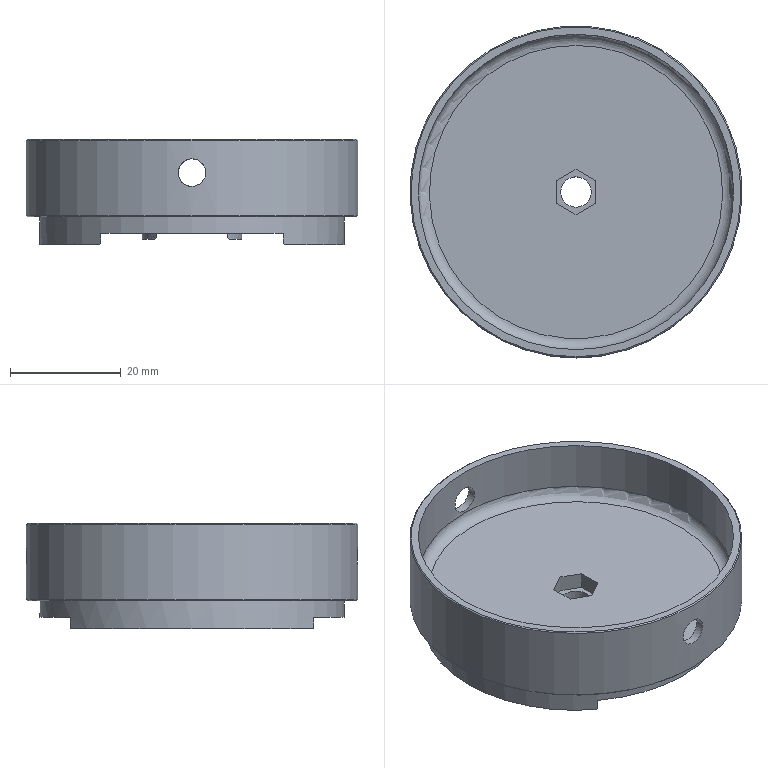NC program | NX | posted with a generic post | part box 60 x 60 x 19 mm
Lines 48 to 904 of 4306:
(ZLEVEL_PROFILE , TOOL : D17R0.8)
N82 T19 M6
N84 G54
N86 G17 G0 G90 X-28.758 Y21.937 S2000 M3
N88 G43 Z30. H19
N90 Z1.5
N92 G94 G1 X-28.558 Y22.222 Z1.482 F1000.
N94 X-27.6 Y23.372 Z1.403
N96 X-26.481 Y24.645 Z1.314
N98 X-25.826 Y25.325 Z1.265
N100 X-24.597 Y26.492 Z1.176
N102 X-24.223 Y26.834 Z1.15
N104 X-21.543 Y29.084 Z0.966
N106 X-18.799 Y30.884 Z0.794
N108 X-18.231 Y31.207 Z0.76
N110 X-16.426 Y32.203 Z0.652
N112 X-14.998 Y32.907 Z0.569
N114 X-11.75 Y34.202 Z0.385
N116 X-10.23 Y34.672 Z0.302
N118 X-9.62 Y34.847 Z0.269
N120 X-6.996 Y35.467 Z0.127
N122 X-6.582 Y35.546 Z0.105
N124 X-3.647 Y35.966 Z-0.05
N126 X-2.061 Y36.105 Z-0.134
N128 X-0.76 Y36.15 Z-0.202
N130 X0.833 Y36.121 Z-0.285
N132 G2 X2.975 Y36.027 R42.264 F2000.
N134 G1 X3.544 Y35.976
N136 X6.299 Y35.597
N138 G2 X9.572 Y34.86 R85.465
N140 X13.67 Y33.451 R44.514
N142 G1 X15.821 Y32.504
N144 G2 X23.134 Y27.813 R40.715
N146 X26.492 Y24.597 R50.528
N148 G1 X26.927 Y24.12
N150 X28.606 Y22.092
N152 X28.636 Y22.064
N154 G2 X33.853 Y12.658 R37.489
N156 G1 X34.674 Y10.225
N158 X34.847 Y9.62
N160 X35.467 Y6.996
N162 X35.546 Y6.582
N164 X35.966 Y3.647
N166 G2 X36.027 Y-2.975 R42.04
N168 G1 X35.976 Y-3.544
N170 X35.597 Y-6.299
N172 G2 X34.86 Y-9.572 R85.504
N174 X27.6 Y-23.372 R37.306
N176 X24.597 Y-26.492 R47.867
N178 G1 X24.223 Y-26.834
N180 X21.742 Y-28.881
N182 G2 X12.658 Y-33.855 R37.588
N184 G1 X12.45 Y-33.922
N186 X10.632 Y-34.531
N188 X10.194 Y-34.683
N190 X9.62 Y-34.847
N192 X6.996 Y-35.467
N194 X6.582 Y-35.546
N196 X3.647 Y-35.966
N198 G2 X-4.886 Y-35.851 R42.264
N200 X-9.572 Y-34.86 R59.819
N202 X-13.67 Y-33.451 R44.514
N204 G1 X-15.821 Y-32.504
N206 G2 X-21.538 Y-29.031 R40.48
N208 G1 X-21.614 Y-28.977
N210 G2 X-24.12 Y-26.927 R58.873
N212 G1 X-24.597 Y-26.492
N214 X-26.492 Y-24.597
N216 X-26.927 Y-24.12
N218 X-28.606 Y-22.092
N220 X-28.636 Y-22.064
N222 G2 X-33.853 Y-12.658 R37.489
N224 G1 X-34.674 Y-10.225
N226 X-34.847 Y-9.62
N228 X-35.467 Y-6.996
N230 X-35.546 Y-6.582
N232 X-35.966 Y-3.647
N234 G2 X-36.027 Y2.975 R42.04
N236 G1 X-35.976 Y3.544
N238 X-35.597 Y6.299
N240 G2 X-34.86 Y9.572 R85.504
N242 X-27.6 Y23.372 R37.306
N244 X-24.597 Y26.492 R47.867
N246 G1 X-24.223 Y26.834
N248 X-21.543 Y29.084
N250 X-18.799 Y30.884
N252 X-18.231 Y31.207
N254 X-16.426 Y32.203
N256 G2 X-10.23 Y34.672 R42.213
N258 G1 X-9.62 Y34.847
N260 X-6.996 Y35.467
N262 X-6.582 Y35.546
N264 X-3.647 Y35.966
N266 G2 X0.833 Y36.121 R42.264
N268 G1 X1.313 Y36.1 Z-0.294
N270 X1.793 Y36.078 Z-0.302
N272 X2.273 Y36.056 Z-0.31
N274 X2.753 Y36.034 Z-0.319
N276 X3.233 Y36.004 Z-0.327
N278 X3.711 Y35.954 Z-0.336
N280 X4.187 Y35.888 Z-0.344
N282 X4.663 Y35.821 Z-0.352
N284 X5.14 Y35.756 Z-0.361
N286 X5.616 Y35.689 Z-0.369
N288 X6.092 Y35.623 Z-0.378
N290 X6.567 Y35.548 Z-0.386
N292 X7.038 Y35.453 Z-0.394
N294 X7.506 Y35.343 Z-0.403
N296 X7.974 Y35.232 Z-0.411
N298 X8.442 Y35.123 Z-0.42
N300 X8.91 Y35.013 Z-0.428
N302 X9.378 Y34.903 Z-0.436
N304 X9.843 Y34.783 Z-0.445
N306 X10.303 Y34.644 Z-0.453
N308 X10.759 Y34.492 Z-0.462
N310 X11.215 Y34.339 Z-0.47
N312 X11.671 Y34.186 Z-0.478
N314 X12.126 Y34.033 Z-0.487
N316 X12.583 Y33.88 Z-0.495
N318 X13.035 Y33.718 Z-0.503
N320 X13.48 Y33.536 Z-0.512
N322 X13.92 Y33.341 Z-0.52
N324 X14.359 Y33.146 Z-0.529
N326 X14.799 Y32.953 Z-0.537
N328 X15.239 Y32.759 Z-0.545
N330 X15.679 Y32.564 Z-0.554
N332 X16.114 Y32.359 Z-0.562
N334 X16.54 Y32.138 Z-0.571
N336 G2 X23.181 Y27.771 R39.763
N338 X26.492 Y24.597 R49.877
N340 G1 X26.927 Y24.12
N342 X28.606 Y22.092
N344 X28.636 Y22.064
N346 G2 X33.922 Y12.451 R36.98
N348 G1 X34.674 Y10.225
N350 X34.847 Y9.62
N352 X35.467 Y6.996
N354 X35.546 Y6.582
N356 X35.966 Y3.647
N358 G2 X36.027 Y-2.975 R41.91
N360 G1 X35.976 Y-3.544
N362 X35.597 Y-6.299
N364 G2 X34.86 Y-9.572 R85.382
N366 X27.597 Y-23.374 R37.295
N368 X24.597 Y-26.492 R47.73
N370 G1 X24.223 Y-26.834
N372 X21.878 Y-28.776
N374 X21.742 Y-28.881
N376 G2 X12.658 Y-33.855 R37.568
N378 G1 X12.45 Y-33.922
N380 X10.632 Y-34.531
N382 X10.194 Y-34.683
N384 X9.62 Y-34.847
N386 X6.996 Y-35.467
N388 X6.582 Y-35.546
N390 X3.647 Y-35.966
N392 G2 X-4.891 Y-35.851 R42.205
N394 X-9.572 Y-34.86 R59.74
N396 X-13.67 Y-33.451 R44.454
N398 G1 X-15.821 Y-32.504
N400 G2 X-21.538 Y-29.031 R39.437
N402 G1 X-21.614 Y-28.977
N404 G2 X-24.12 Y-26.927 R58.37
N406 G1 X-24.597 Y-26.492
N408 X-26.492 Y-24.597
N410 X-26.927 Y-24.12
N412 X-28.606 Y-22.092
N414 X-28.636 Y-22.064
N416 G2 X-33.922 Y-12.451 R36.98
N418 G1 X-34.674 Y-10.225
N420 X-34.847 Y-9.62
N422 X-35.467 Y-6.996
N424 X-35.546 Y-6.582
N426 X-35.966 Y-3.647
N428 G2 X-36.027 Y2.975 R41.91
N430 G1 X-35.976 Y3.544
N432 X-35.597 Y6.299
N434 G2 X-34.86 Y9.572 R85.382
N436 X-27.597 Y23.374 R37.295
N438 X-24.597 Y26.492 R47.73
N440 G1 X-24.223 Y26.834
N442 X-21.543 Y29.084
N444 X-18.799 Y30.884
N446 X-18.231 Y31.207
N448 X-16.426 Y32.203
N450 G2 X-10.23 Y34.672 R42.158
N452 G1 X-9.62 Y34.847
N454 X-6.996 Y35.467
N456 X-6.582 Y35.546
N458 X-3.647 Y35.966
N460 G2 X0.833 Y36.121 R42.205
N462 G1 X1.313 Y36.1 Z-0.579
N464 X1.793 Y36.078 Z-0.587
N466 X2.273 Y36.056 Z-0.596
N468 X2.753 Y36.033 Z-0.604
N470 X3.233 Y36.004 Z-0.613
N472 X3.711 Y35.955 Z-0.621
N474 X4.187 Y35.889 Z-0.629
N476 X4.663 Y35.822 Z-0.638
N478 X5.14 Y35.756 Z-0.646
N480 X5.616 Y35.689 Z-0.654
N482 X6.092 Y35.623 Z-0.663
N484 X6.567 Y35.548 Z-0.671
N486 X7.038 Y35.453 Z-0.68
N488 X7.506 Y35.343 Z-0.688
N490 X7.974 Y35.233 Z-0.696
N492 X8.442 Y35.123 Z-0.705
N494 X8.91 Y35.012 Z-0.713
N496 X9.378 Y34.903 Z-0.722
N498 X9.843 Y34.784 Z-0.73
N500 X10.303 Y34.644 Z-0.738
N502 X10.759 Y34.492 Z-0.747
N504 X11.215 Y34.338 Z-0.755
N506 X11.671 Y34.186 Z-0.764
N508 X12.127 Y34.033 Z-0.772
N510 X12.583 Y33.881 Z-0.78
N512 X13.035 Y33.718 Z-0.789
N514 X13.48 Y33.536 Z-0.797
N516 X13.92 Y33.341 Z-0.806
N518 X14.36 Y33.146 Z-0.814
N520 X14.799 Y32.953 Z-0.822
N522 X15.239 Y32.758 Z-0.831
N524 X15.679 Y32.565 Z-0.839
N526 X16.114 Y32.36 Z-0.847
N528 X16.54 Y32.137 Z-0.856
N530 X18.782 Y30.884
N532 G2 X21.423 Y29.118 R104.416
N534 X21.879 Y-28.777 R36.15
N536 G1 X21.742 Y-28.881
N538 G2 X21.432 Y-29.112 R36.15
N540 X18.784 Y-30.884 R93.01
N542 X12.658 Y-33.855 R39.61
N544 G1 X12.45 Y-33.922
N546 X10.632 Y-34.531
N548 X10.194 Y-34.683
N550 G2 X9.572 Y-34.86 R36.15
N552 G1 X6.996 Y-35.467
N554 G2 X6.299 Y-35.597 R36.15
N556 G1 X6.266 Y-35.595
N558 X3.698 Y-35.953
N560 X3.647 Y-35.966
N562 G2 X2.975 Y-36.027 R36.15
N564 X-2.975 Y-36.027 R44.388
N566 X-6.996 Y-35.467 R36.15
N568 G1 X-9.572 Y-34.86
N570 G2 X-10.225 Y-34.674 R36.15
N572 X-15.821 Y-32.504 R44.549
N574 X-20.375 Y-29.861 R36.15
N576 G1 X-21.595 Y-28.991
N578 G2 X-20.993 Y29.432 R36.152
N580 G1 X-20.343 Y29.883
N582 G2 X-18.515 Y31.048 R36.15
N584 G1 X-16.426 Y32.203
N586 G2 X-15.821 Y32.504 R36.15
N588 X-10.23 Y34.672 R44.561
N590 X-9.572 Y34.86 R36.15
N592 G1 X-6.996 Y35.467
N594 G2 X-6.299 Y35.597 R36.15
N596 G1 X-6.266 Y35.595
N598 X-3.698 Y35.953
N600 X-3.647 Y35.966
N602 G2 X-2.975 Y36.027 R36.15
N604 X0.833 Y36.119 R44.388
N606 G1 X1.313 Y36.1 Z-0.864
N608 X1.793 Y36.079 Z-0.873
N610 X2.273 Y36.056 Z-0.881
N612 X2.753 Y36.034 Z-0.889
N614 X3.233 Y36.005 Z-0.898
N616 X3.711 Y35.955 Z-0.906
N618 X4.187 Y35.888 Z-0.915
N620 X4.663 Y35.822 Z-0.923
N622 X5.139 Y35.756 Z-0.931
N624 X5.615 Y35.689 Z-0.94
N626 X6.091 Y35.623 Z-0.948
N628 X6.566 Y35.549 Z-0.957
N630 X7.037 Y35.453 Z-0.965
N632 X7.505 Y35.343 Z-0.973
N634 X7.973 Y35.233 Z-0.982
N636 X8.44 Y35.123 Z-0.99
N638 X8.909 Y35.014 Z-0.999
N640 X9.377 Y34.903 Z-1.007
N642 X9.842 Y34.784 Z-1.015
N644 X10.302 Y34.645 Z-1.024
N646 X10.758 Y34.492 Z-1.032
N648 X11.214 Y34.34 Z-1.04
N650 X11.669 Y34.187 Z-1.049
N652 X12.125 Y34.033 Z-1.057
N654 X12.581 Y33.881 Z-1.066
N656 X13.034 Y33.719 Z-1.074
N658 X13.479 Y33.536 Z-1.082
N660 X13.919 Y33.342 Z-1.091
N662 X14.358 Y33.147 Z-1.099
N664 X14.798 Y32.953 Z-1.108
N666 X15.238 Y32.759 Z-1.116
N668 X15.678 Y32.565 Z-1.124
N670 X16.113 Y32.36 Z-1.133
N672 X16.541 Y32.142 Z-1.141
N674 G2 X21.423 Y29.118 R41.074
N676 X21.432 Y-29.112 R36.15
N678 X15.695 Y-32.559 R39.486
N680 X10.194 Y-34.683 R41.1
N682 X9.572 Y-34.86 R36.15
N684 G1 X6.996 Y-35.467
N686 G2 X6.299 Y-35.597 R36.15
N688 G1 X6.266 Y-35.595
N690 X3.698 Y-35.954
N692 X3.647 Y-35.966
N694 G2 X2.975 Y-36.027 R36.15
N696 X-2.975 Y-36.027 R44.22
N698 X-6.996 Y-35.467 R36.15
N700 G1 X-9.572 Y-34.86
N702 G2 X-10.225 Y-34.674 R36.15
N704 X-15.821 Y-32.504 R44.497
N706 X-16.421 Y-32.205 R36.15
N708 X-21.509 Y-29.052 R41.028
N710 X-21.69 Y-28.92 R8.65
N712 X-20.993 Y29.432 R36.152
N714 G1 X-20.343 Y29.883
N716 G2 X-18.515 Y31.048 R36.15
N718 G1 X-16.426 Y32.203
N720 G2 X-15.821 Y32.504 R36.15
N722 X-10.23 Y34.672 R44.218
N724 X-9.572 Y34.86 R36.15
N726 G1 X-6.996 Y35.467
N728 G2 X-6.299 Y35.597 R36.15
N730 G1 X-6.266 Y35.595
N732 X-3.698 Y35.954
N734 X-3.647 Y35.966
N736 G2 X-2.975 Y36.027 R36.15
N738 X0.833 Y36.12 R44.22
N740 G1 X1.313 Y36.1 Z-1.15
N742 X1.793 Y36.078 Z-1.158
N744 X2.273 Y36.056 Z-1.166
N746 X2.753 Y36.034 Z-1.175
N748 X3.233 Y36.005 Z-1.183
N750 X3.711 Y35.954 Z-1.192
N752 X4.187 Y35.889 Z-1.2
N754 X4.663 Y35.822 Z-1.208
N756 X5.139 Y35.756 Z-1.217
N758 X5.615 Y35.689 Z-1.225
N760 X6.091 Y35.622 Z-1.233
N762 X6.566 Y35.549 Z-1.242
N764 X7.037 Y35.454 Z-1.25
N766 X7.505 Y35.343 Z-1.259
N768 X7.973 Y35.234 Z-1.267
N770 X8.441 Y35.123 Z-1.275
N772 X8.909 Y35.014 Z-1.284
N774 X9.377 Y34.903 Z-1.292
N776 X9.842 Y34.784 Z-1.301
N778 X10.302 Y34.645 Z-1.309
N780 X10.758 Y34.492 Z-1.317
N782 X11.214 Y34.34 Z-1.326
N784 X11.669 Y34.186 Z-1.334
N786 X12.125 Y34.033 Z-1.343
N788 X12.581 Y33.881 Z-1.351
N790 X13.034 Y33.719 Z-1.359
N792 X13.479 Y33.536 Z-1.368
N794 X13.919 Y33.342 Z-1.376
N796 X14.359 Y33.147 Z-1.385
N798 X14.798 Y32.953 Z-1.393
N800 X15.238 Y32.759 Z-1.401
N802 X15.678 Y32.565 Z-1.41
N804 X16.113 Y32.36 Z-1.418
N806 X16.541 Y32.142 Z-1.426
N808 G2 X21.423 Y29.118 R41.002
N810 X21.432 Y-29.112 R36.15
N812 X18.733 Y-30.916 R88.63
N814 X10.194 Y-34.683 R38.805
N816 X9.572 Y-34.86 R36.15
N818 G1 X6.996 Y-35.467
N820 G2 X6.299 Y-35.597 R36.15
N822 G1 X6.266 Y-35.596
N824 X3.698 Y-35.954
N826 X3.647 Y-35.966
N828 G2 X2.975 Y-36.027 R36.15
N830 X-2.975 Y-36.027 R44.054
N832 X-6.996 Y-35.467 R36.15
N834 G1 X-9.572 Y-34.86
N836 G2 X-10.225 Y-34.674 R36.15
N838 X-15.821 Y-32.504 R44.446
N840 X-16.421 Y-32.205 R36.15
N842 X-21.509 Y-29.052 R41.028
N844 X-21.69 Y-28.92 R8.65
N846 X-20.993 Y29.432 R36.152
N848 G1 X-20.343 Y29.883
N850 G2 X-18.515 Y31.048 R36.15
N852 G1 X-16.426 Y32.203
N854 G2 X-15.821 Y32.504 R36.15
N856 X-10.23 Y34.672 R44.119
N858 X-9.572 Y34.86 R36.15
N860 G1 X-6.996 Y35.467
N862 G2 X-6.299 Y35.597 R36.15
N864 G1 X-6.266 Y35.596
N866 X-3.698 Y35.954
N868 X-3.647 Y35.966
N870 G2 X-2.975 Y36.027 R36.15
N872 X0.833 Y36.12 R44.054
N874 G1 X1.313 Y36.101 Z-1.435
N876 X1.793 Y36.078 Z-1.443
N878 X2.273 Y36.056 Z-1.452
N880 X2.753 Y36.035 Z-1.46
N882 X3.233 Y36.005 Z-1.468
N884 X3.711 Y35.955 Z-1.477
N886 X4.187 Y35.889 Z-1.485
N888 X4.663 Y35.822 Z-1.494
N890 X5.139 Y35.756 Z-1.502
N892 X5.615 Y35.689 Z-1.51
N894 X6.091 Y35.623 Z-1.519
N896 X6.566 Y35.549 Z-1.527
N898 X7.037 Y35.454 Z-1.536
N900 X7.505 Y35.343 Z-1.544
N902 X7.973 Y35.234 Z-1.552
N904 X8.441 Y35.123 Z-1.561
N906 X8.909 Y35.013 Z-1.569
N908 X9.377 Y34.903 Z-1.578
N910 X9.842 Y34.784 Z-1.586
N912 X10.302 Y34.645 Z-1.594
N914 X10.758 Y34.492 Z-1.603
N916 X11.213 Y34.339 Z-1.611
N918 X11.669 Y34.187 Z-1.619
N920 X12.125 Y34.034 Z-1.628
N922 X12.581 Y33.881 Z-1.636
N924 X13.034 Y33.719 Z-1.645
N926 X13.479 Y33.536 Z-1.653
N928 X13.919 Y33.342 Z-1.661
N930 X14.359 Y33.147 Z-1.67
N932 X14.799 Y32.953 Z-1.678
N934 X15.238 Y32.759 Z-1.687
N936 X15.678 Y32.565 Z-1.695
N938 X16.113 Y32.36 Z-1.703
N940 X16.541 Y32.142 Z-1.712
N942 G2 X21.423 Y29.118 R40.93
N944 X21.432 Y-29.112 R36.15
N946 X18.733 Y-30.917 R88.3
N948 X10.194 Y-34.683 R38.697
N950 X9.572 Y-34.86 R36.15
N952 G1 X6.996 Y-35.467
N954 G2 X6.299 Y-35.597 R36.15
N956 G1 X6.266 Y-35.596
N958 X3.698 Y-35.954
N960 X3.647 Y-35.966
N962 G2 X2.975 Y-36.027 R36.15
N964 X-2.975 Y-36.027 R43.889
N966 X-6.996 Y-35.467 R36.15
N968 G1 X-9.572 Y-34.86
N970 G2 X-10.225 Y-34.674 R36.15
N972 X-15.821 Y-32.504 R44.395
N974 X-16.421 Y-32.205 R36.15
N976 X-21.509 Y-29.052 R41.028
N978 X-21.69 Y-28.92 R8.65
N980 X-20.993 Y29.432 R36.152
N982 G1 X-20.343 Y29.883
N984 G2 X-18.515 Y31.048 R36.15
N986 G1 X-16.426 Y32.203
N988 G2 X-15.821 Y32.504 R36.15
N990 X-12.658 Y33.853 R69.78
N992 G1 X-10.23 Y34.672
N994 G2 X-9.572 Y34.86 R36.15
N996 G1 X-6.996 Y35.467
N998 G2 X-6.299 Y35.597 R36.15
N1000 G1 X-6.266 Y35.596
N1002 X-3.698 Y35.954
N1004 X-3.647 Y35.966
N1006 G2 X-2.975 Y36.027 R36.15
N1008 X0.833 Y36.12 R43.889
N1010 G1 X1.313 Y36.101 Z-1.72
N1012 X1.793 Y36.079 Z-1.729
N1014 X2.273 Y36.057 Z-1.737
N1016 X2.753 Y36.034 Z-1.745
N1018 X3.233 Y36.005 Z-1.754
N1020 X3.711 Y35.955 Z-1.762
N1022 X4.187 Y35.888 Z-1.771
N1024 X4.663 Y35.822 Z-1.779
N1026 X5.139 Y35.755 Z-1.787
N1028 X5.615 Y35.689 Z-1.796
N1030 X6.091 Y35.623 Z-1.804
N1032 X6.566 Y35.549 Z-1.812
N1034 X7.037 Y35.454 Z-1.821
N1036 X7.505 Y35.343 Z-1.829
N1038 X7.973 Y35.234 Z-1.838
N1040 X8.441 Y35.123 Z-1.846
N1042 X8.909 Y35.013 Z-1.854
N1044 X9.377 Y34.903 Z-1.863
N1046 X9.842 Y34.784 Z-1.871
N1048 X10.302 Y34.645 Z-1.88
N1050 X10.758 Y34.492 Z-1.888
N1052 X11.214 Y34.339 Z-1.896
N1054 X11.67 Y34.187 Z-1.905
N1056 X12.125 Y34.034 Z-1.913
N1058 X12.581 Y33.881 Z-1.922
N1060 X13.034 Y33.719 Z-1.93
N1062 X13.479 Y33.536 Z-1.938
N1064 X13.919 Y33.342 Z-1.947
N1066 X14.359 Y33.148 Z-1.955
N1068 X14.799 Y32.954 Z-1.963
N1070 X15.238 Y32.759 Z-1.972
N1072 X15.678 Y32.565 Z-1.98
N1074 X16.113 Y32.36 Z-1.989
N1076 X16.541 Y32.142 Z-1.997
N1078 G2 X21.423 Y29.118 R40.859
N1080 X21.432 Y-29.112 R36.15
N1082 X18.733 Y-30.917 R87.978
N1084 X10.194 Y-34.683 R38.591
N1086 X9.572 Y-34.86 R36.15
N1088 G1 X6.996 Y-35.467
N1090 G2 X6.299 Y-35.597 R36.15
N1092 G1 X6.266 Y-35.596
N1094 X3.698 Y-35.954
N1096 X3.647 Y-35.966
N1098 G2 X2.975 Y-36.027 R36.15
N1100 X-2.975 Y-36.027 R43.728
N1102 X-6.996 Y-35.467 R36.15
N1104 G1 X-9.572 Y-34.86
N1106 G2 X-10.225 Y-34.674 R36.15
N1108 X-15.821 Y-32.504 R44.344
N1110 X-16.421 Y-32.205 R36.15
N1112 X-21.509 Y-29.052 R41.028
N1114 X-21.69 Y-28.92 R8.65
N1116 X-20.994 Y29.432 R36.152
N1118 G1 X-20.343 Y29.883
N1120 G2 X-18.515 Y31.048 R36.15
N1122 G1 X-16.426 Y32.203
N1124 G2 X-15.821 Y32.504 R36.15
N1126 X-12.658 Y33.853 R69.614
N1128 G1 X-10.23 Y34.672
N1130 G2 X-9.572 Y34.86 R36.15
N1132 G1 X-6.996 Y35.467
N1134 G2 X-6.299 Y35.597 R36.15
N1136 G1 X-6.266 Y35.596
N1138 X-3.698 Y35.954
N1140 X-3.647 Y35.966
N1142 G2 X-2.975 Y36.027 R36.15
N1144 X0.833 Y36.121 R43.728
N1146 G1 X1.313 Y36.101 Z-2.005
N1148 X1.793 Y36.079 Z-2.014
N1150 X2.273 Y36.056 Z-2.022
N1152 X2.753 Y36.034 Z-2.031
N1154 X3.233 Y36.005 Z-2.039
N1156 X3.711 Y35.955 Z-2.047
N1158 X4.187 Y35.889 Z-2.056
N1160 X4.663 Y35.822 Z-2.064
N1162 X5.139 Y35.756 Z-2.073
N1164 X5.615 Y35.69 Z-2.081
N1166 X6.091 Y35.623 Z-2.089
N1168 X6.566 Y35.549 Z-2.098
N1170 X7.037 Y35.454 Z-2.106
N1172 X7.505 Y35.344 Z-2.115
N1174 X7.973 Y35.233 Z-2.123
N1176 X8.441 Y35.123 Z-2.131
N1178 X8.909 Y35.013 Z-2.14
N1180 X9.377 Y34.904 Z-2.148
N1182 X9.842 Y34.784 Z-2.156
N1184 X10.302 Y34.645 Z-2.165
N1186 X10.758 Y34.492 Z-2.173
N1188 X11.214 Y34.339 Z-2.182
N1190 X11.669 Y34.186 Z-2.19
N1192 X12.125 Y34.034 Z-2.198
N1194 X12.581 Y33.881 Z-2.207
N1196 X13.034 Y33.719 Z-2.215
N1198 X13.479 Y33.536 Z-2.224
N1200 X13.919 Y33.341 Z-2.232
N1202 X14.359 Y33.147 Z-2.24
N1204 X14.799 Y32.954 Z-2.249
N1206 X15.238 Y32.759 Z-2.257
N1208 X15.678 Y32.565 Z-2.266
N1210 X16.113 Y32.36 Z-2.274
N1212 X16.541 Y32.142 Z-2.282
N1214 G2 X21.423 Y29.118 R40.787
N1216 X21.432 Y-29.112 R36.15
N1218 X18.733 Y-30.917 R87.649
N1220 X10.194 Y-34.683 R38.482
N1222 X9.572 Y-34.86 R36.15
N1224 G1 X6.996 Y-35.467
N1226 G2 X6.299 Y-35.597 R36.15
N1228 G1 X6.266 Y-35.596
N1230 X3.698 Y-35.954
N1232 X3.647 Y-35.966
N1234 G2 X2.975 Y-36.027 R36.15
N1236 X-2.975 Y-36.027 R43.563
N1238 X-6.996 Y-35.467 R36.15
N1240 G1 X-9.572 Y-34.86
N1242 G2 X-10.225 Y-34.674 R36.15
N1244 X-15.821 Y-32.504 R44.292
N1246 X-16.421 Y-32.205 R36.15
N1248 X-21.509 Y-29.052 R41.028
N1250 X-21.69 Y-28.92 R8.65
N1252 X-20.994 Y29.433 R36.153
N1254 G1 X-20.343 Y29.883
N1256 G2 X-18.515 Y31.048 R36.15
N1258 G1 X-16.426 Y32.203
N1260 G2 X-15.821 Y32.504 R36.15
N1262 X-10.23 Y34.672 R43.824
N1264 X-9.572 Y34.86 R36.15
N1266 G1 X-6.996 Y35.467
N1268 G2 X-6.299 Y35.597 R36.15
N1270 G1 X-6.266 Y35.596
N1272 X-3.698 Y35.954
N1274 X-3.647 Y35.966
N1276 G2 X-2.975 Y36.027 R36.15
N1278 X0.833 Y36.121 R43.563
N1280 G1 X1.313 Y36.101 Z-2.291
N1282 X1.793 Y36.079 Z-2.299
N1284 X2.273 Y36.056 Z-2.308
N1286 X2.753 Y36.034 Z-2.316
N1288 X3.233 Y36.005 Z-2.324
N1290 X3.711 Y35.955 Z-2.333
N1292 X4.187 Y35.889 Z-2.341
N1294 X4.663 Y35.823 Z-2.349
N1296 X5.139 Y35.756 Z-2.358
N1298 X5.616 Y35.69 Z-2.366
N1300 X6.091 Y35.623 Z-2.375
N1302 X6.566 Y35.549 Z-2.383
N1304 X7.037 Y35.454 Z-2.391
N1306 X7.505 Y35.344 Z-2.4
N1308 X7.973 Y35.233 Z-2.408
N1310 X8.441 Y35.123 Z-2.417
N1312 X8.909 Y35.013 Z-2.425
N1314 X9.377 Y34.904 Z-2.433
N1316 X9.842 Y34.784 Z-2.442
N1318 X10.302 Y34.645 Z-2.45
N1320 X10.758 Y34.492 Z-2.459
N1322 X11.214 Y34.339 Z-2.467
N1324 X11.669 Y34.187 Z-2.475
N1326 X12.125 Y34.034 Z-2.484
N1328 X12.581 Y33.881 Z-2.492
N1330 X13.034 Y33.718 Z-2.501
N1332 X13.479 Y33.537 Z-2.509
N1334 X13.919 Y33.341 Z-2.517
N1336 X14.359 Y33.148 Z-2.526
N1338 X14.799 Y32.954 Z-2.534
N1340 X15.238 Y32.759 Z-2.542
N1342 X15.678 Y32.565 Z-2.551
N1344 X16.113 Y32.36 Z-2.559
N1346 X16.541 Y32.142 Z-2.568
N1348 G2 X21.423 Y29.118 R40.715
N1350 X21.432 Y-29.112 R36.15
N1352 X18.733 Y-30.917 R87.327
N1354 X10.194 Y-34.683 R38.376
N1356 X9.572 Y-34.86 R36.15
N1358 G1 X6.996 Y-35.467
N1360 G2 X6.299 Y-35.597 R36.15
N1362 G1 X6.266 Y-35.596
N1364 X3.698 Y-35.954
N1366 X3.647 Y-35.966
N1368 G2 X2.975 Y-36.027 R36.15
N1370 X-2.975 Y-36.027 R43.784
N1372 X-6.996 Y-35.467 R36.15
N1374 G1 X-9.572 Y-34.86
N1376 G2 X-10.225 Y-34.674 R36.15
N1378 X-15.821 Y-32.504 R44.241
N1380 X-16.421 Y-32.205 R36.15
N1382 X-21.509 Y-29.052 R41.028
N1384 X-21.69 Y-28.92 R8.65
N1386 X-20.994 Y29.433 R36.153
N1388 G1 X-20.343 Y29.883
N1390 G2 X-18.515 Y31.048 R36.15
N1392 G1 X-16.426 Y32.203
N1394 G2 X-15.821 Y32.504 R36.15
N1396 X-12.658 Y33.853 R68.821
N1398 G1 X-10.23 Y34.672
N1400 G2 X-9.572 Y34.86 R36.15
N1402 G1 X-6.996 Y35.467
N1404 G2 X-6.299 Y35.597 R36.15
N1406 G1 X-6.266 Y35.596
N1408 X-3.698 Y35.954
N1410 X-3.647 Y35.966
N1412 G2 X-2.975 Y36.027 R36.15
N1414 X0.833 Y36.121 R43.784
N1416 G1 X1.313 Y36.101 Z-2.576
N1418 X1.793 Y36.079 Z-2.584
N1420 X2.273 Y36.056 Z-2.593
N1422 X2.753 Y36.034 Z-2.601
N1424 X3.233 Y36.005 Z-2.61
N1426 X3.711 Y35.955 Z-2.618
N1428 X4.187 Y35.888 Z-2.626
N1430 X4.664 Y35.83 Z-2.635
N1432 X5.141 Y35.767 Z-2.643
N1434 X5.617 Y35.697 Z-2.652
N1436 X6.091 Y35.623 Z-2.66
N1438 X6.566 Y35.549 Z-2.668
N1440 X7.037 Y35.454 Z-2.677
N1442 X7.507 Y35.353 Z-2.685
N1444 X7.977 Y35.252 Z-2.694
N1446 X8.446 Y35.143 Z-2.702
N1448 X8.912 Y35.029 Z-2.71
N1450 X9.378 Y34.908 Z-2.719
N1452 X9.842 Y34.784 Z-2.727
N1454 X10.303 Y34.648 Z-2.735
N1456 X10.763 Y34.508 Z-2.744
N1458 X11.222 Y34.363 Z-2.752
N1460 X11.678 Y34.211 Z-2.761
N1462 X12.132 Y34.053 Z-2.769
N1464 X12.584 Y33.889 Z-2.777
N1466 X13.034 Y33.718 Z-2.786
N1468 X13.481 Y33.542 Z-2.794
N1470 X13.927 Y33.36 Z-2.803
N1472 X14.369 Y33.172 Z-2.811
N1474 X14.809 Y32.977 Z-2.819
N1476 X15.246 Y32.778 Z-2.828
N1478 X15.681 Y32.572 Z-2.836
N1480 X16.113 Y32.36 Z-2.845
N1482 X16.542 Y32.143 Z-2.853
N1484 G2 X0.833 Y36.14 R-36.15
N1486 G1 X1.314 Y36.126 Z-2.861
N1488 X1.794 Y36.105 Z-2.87
N1490 X2.274 Y36.078 Z-2.878
N1492 X2.754 Y36.045 Z-2.887
N1494 X3.233 Y36.005 Z-2.895
N1496 X3.711 Y35.959 Z-2.903
N1498 X4.189 Y35.906 Z-2.912
N1500 X4.666 Y35.848 Z-2.92
N1502 X5.142 Y35.782 Z-2.928
N1504 X5.618 Y35.711 Z-2.937
N1506 X6.092 Y35.633 Z-2.945
N1508 X6.565 Y35.549 Z-2.954
N1510 X7.037 Y35.458 Z-2.962
N1512 X7.508 Y35.362 Z-2.97
N1514 X7.978 Y35.259 Z-2.979
N1516 X8.446 Y35.149 Z-2.987
N1518 X8.913 Y35.034 Z-2.996
N1520 X9.378 Y34.912 Z-3.004
N1522 X9.841 Y34.785 Z-3.012
N1524 X10.303 Y34.651 Z-3.021
N1526 X10.763 Y34.511 Z-3.029
N1528 X11.221 Y34.364 Z-3.038
N1530 X11.677 Y34.212 Z-3.046
N1532 X12.131 Y34.054 Z-3.054
N1534 X12.582 Y33.89 Z-3.063
N1536 X13.032 Y33.719 Z-3.071
N1538 X13.479 Y33.543 Z-3.079
N1540 X13.924 Y33.361 Z-3.088
N1542 X14.366 Y33.173 Z-3.096
N1544 X14.806 Y32.979 Z-3.105
N1546 X15.243 Y32.779 Z-3.113
N1548 X15.678 Y32.573 Z-3.121
N1550 X16.11 Y32.362 Z-3.13
N1552 X16.539 Y32.145 Z-3.138
N1554 G2 X0.833 Y36.14 R-36.15
N1556 G1 X1.314 Y36.126 Z-3.147
N1558 X1.794 Y36.105 Z-3.155
N1560 X2.274 Y36.078 Z-3.163
N1562 X2.754 Y36.045 Z-3.172
N1564 X3.233 Y36.005 Z-3.18
N1566 X3.711 Y35.959 Z-3.189
N1568 X4.189 Y35.906 Z-3.197
N1570 X4.666 Y35.848 Z-3.205
N1572 X5.142 Y35.782 Z-3.214
N1574 X5.618 Y35.711 Z-3.222
N1576 X6.092 Y35.633 Z-3.231
N1578 X6.565 Y35.549 Z-3.239
N1580 X7.037 Y35.458 Z-3.247
N1582 X7.508 Y35.362 Z-3.256
N1584 X7.978 Y35.259 Z-3.264
N1586 X8.446 Y35.149 Z-3.272
N1588 X8.913 Y35.034 Z-3.281
N1590 X9.378 Y34.912 Z-3.289
N1592 X9.841 Y34.785 Z-3.298
N1594 X10.303 Y34.651 Z-3.306
N1596 X10.763 Y34.511 Z-3.314
N1598 X11.221 Y34.364 Z-3.323
N1600 X11.677 Y34.212 Z-3.331
N1602 X12.131 Y34.054 Z-3.34
N1604 X12.582 Y33.89 Z-3.348
N1606 X13.032 Y33.719 Z-3.356
N1608 X13.479 Y33.543 Z-3.365
N1610 X13.924 Y33.361 Z-3.373
N1612 X14.366 Y33.173 Z-3.382
N1614 X14.806 Y32.979 Z-3.39
N1616 X15.243 Y32.779 Z-3.398
N1618 X15.678 Y32.573 Z-3.407
N1620 X16.11 Y32.362 Z-3.415
N1622 X16.539 Y32.145 Z-3.424
N1624 G2 X0.833 Y36.14 R-36.15
N1626 G1 X1.314 Y36.126 Z-3.432
N1628 X1.794 Y36.105 Z-3.44
N1630 X2.274 Y36.078 Z-3.449
N1632 X2.754 Y36.045 Z-3.457
N1634 X3.233 Y36.005 Z-3.465
N1636 X3.711 Y35.959 Z-3.474
N1638 X4.189 Y35.906 Z-3.482
N1640 X4.666 Y35.848 Z-3.491
N1642 X5.142 Y35.782 Z-3.499
N1644 X5.618 Y35.711 Z-3.507
N1646 X6.092 Y35.633 Z-3.516
N1648 X6.565 Y35.549 Z-3.524
N1650 X7.037 Y35.458 Z-3.533
N1652 X7.508 Y35.362 Z-3.541
N1654 X7.978 Y35.259 Z-3.549
N1656 X8.446 Y35.149 Z-3.558
N1658 X8.913 Y35.034 Z-3.566
N1660 X9.378 Y34.912 Z-3.575
N1662 X9.841 Y34.785 Z-3.583
N1664 X10.303 Y34.651 Z-3.591
N1666 X10.763 Y34.511 Z-3.6
N1668 X11.221 Y34.364 Z-3.608
N1670 X11.677 Y34.212 Z-3.617
N1672 X12.131 Y34.054 Z-3.625
N1674 X12.582 Y33.89 Z-3.633
N1676 X13.032 Y33.719 Z-3.642
N1678 X13.479 Y33.543 Z-3.65
N1680 X13.924 Y33.361 Z-3.658
N1682 X14.366 Y33.173 Z-3.667
N1684 X14.806 Y32.979 Z-3.675
N1686 X15.243 Y32.779 Z-3.684
N1688 X15.678 Y32.573 Z-3.692
N1690 X16.11 Y32.362 Z-3.7
N1692 X16.539 Y32.145 Z-3.709
N1694 G2 X0.833 Y36.14 R-36.15
N1696 G1 X1.314 Y36.126 Z-3.717
N1698 X1.794 Y36.105 Z-3.726
N1700 X2.274 Y36.078 Z-3.734
N1702 X2.754 Y36.045 Z-3.742
N1704 X3.233 Y36.005 Z-3.751
N1706 X3.711 Y35.959 Z-3.759
N1708 X4.189 Y35.906 Z-3.768
N1710 X4.666 Y35.848 Z-3.776
N1712 X5.142 Y35.782 Z-3.784
N1714 X5.618 Y35.711 Z-3.793
N1716 X6.092 Y35.633 Z-3.801
N1718 X6.565 Y35.549 Z-3.81
N1720 X7.037 Y35.458 Z-3.818
N1722 X7.508 Y35.362 Z-3.826
N1724 X7.978 Y35.259 Z-3.835
N1726 X8.446 Y35.149 Z-3.843
N1728 X8.913 Y35.034 Z-3.851
N1730 X9.378 Y34.912 Z-3.86
N1732 X9.841 Y34.785 Z-3.868
N1734 X10.303 Y34.651 Z-3.877
N1736 X10.763 Y34.511 Z-3.885
N1738 X11.221 Y34.364 Z-3.893
N1740 X11.677 Y34.212 Z-3.902
N1742 X12.131 Y34.054 Z-3.91
N1744 X12.582 Y33.89 Z-3.919
N1746 X13.032 Y33.719 Z-3.927
N1748 X13.479 Y33.543 Z-3.935
N1750 X13.924 Y33.361 Z-3.944
N1752 X14.366 Y33.173 Z-3.952
N1754 X14.806 Y32.979 Z-3.961
N1756 X15.243 Y32.779 Z-3.969
N1758 X15.678 Y32.573 Z-3.977
N1760 X16.11 Y32.362 Z-3.986
N1762 X16.539 Y32.145 Z-3.994
N1764 G2 X0.833 Y36.14 R-36.15
N1766 G1 X1.314 Y36.126 Z-4.003
N1768 X1.794 Y36.105 Z-4.011
N1770 X2.274 Y36.078 Z-4.019
N1772 X2.754 Y36.045 Z-4.028
N1774 X3.233 Y36.005 Z-4.036
N1776 X3.711 Y35.959 Z-4.044
N1778 X4.189 Y35.906 Z-4.053
N1780 X4.666 Y35.848 Z-4.061
N1782 X5.142 Y35.782 Z-4.07
N1784 X5.618 Y35.711 Z-4.078
N1786 X6.092 Y35.633 Z-4.086
N1788 X6.565 Y35.549 Z-4.095